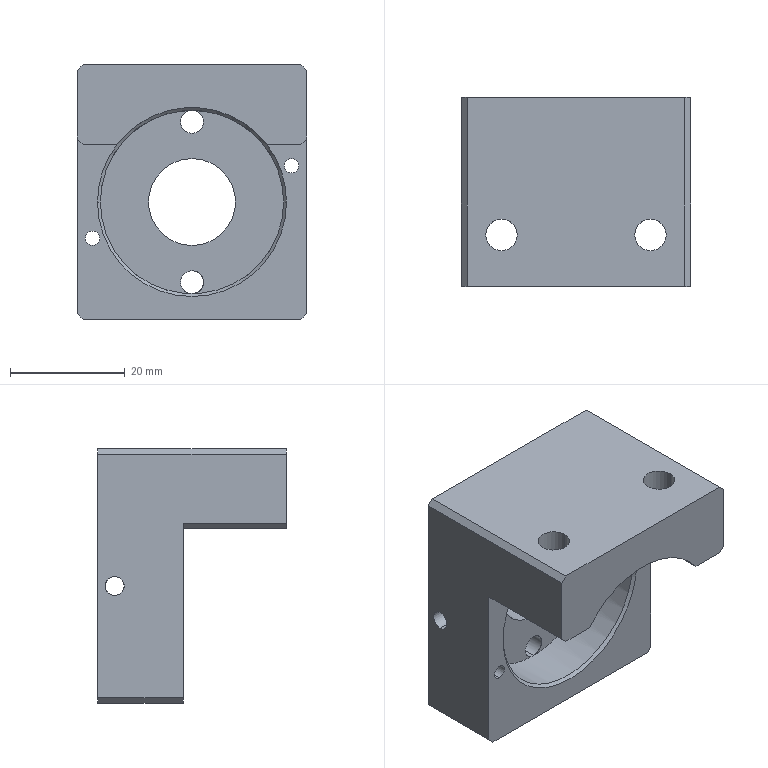Part | STEP file | PN_0001 Drive Bearing Housing | 1 solid | 45 faces | box 40 x 33 x 44.5 mm | volume 24608 mm3 | cylinder 25 | plane 18 | cone 2 | commonest cylinder face diameters 2.5 x4 3.3 x4 4 x4 5.5 x4 10 x4 15.2 x2